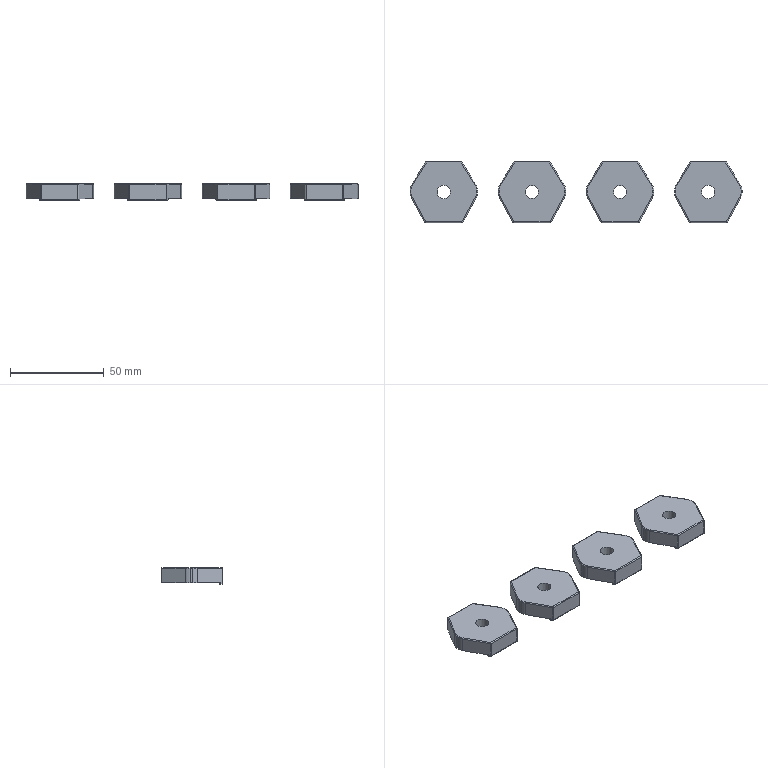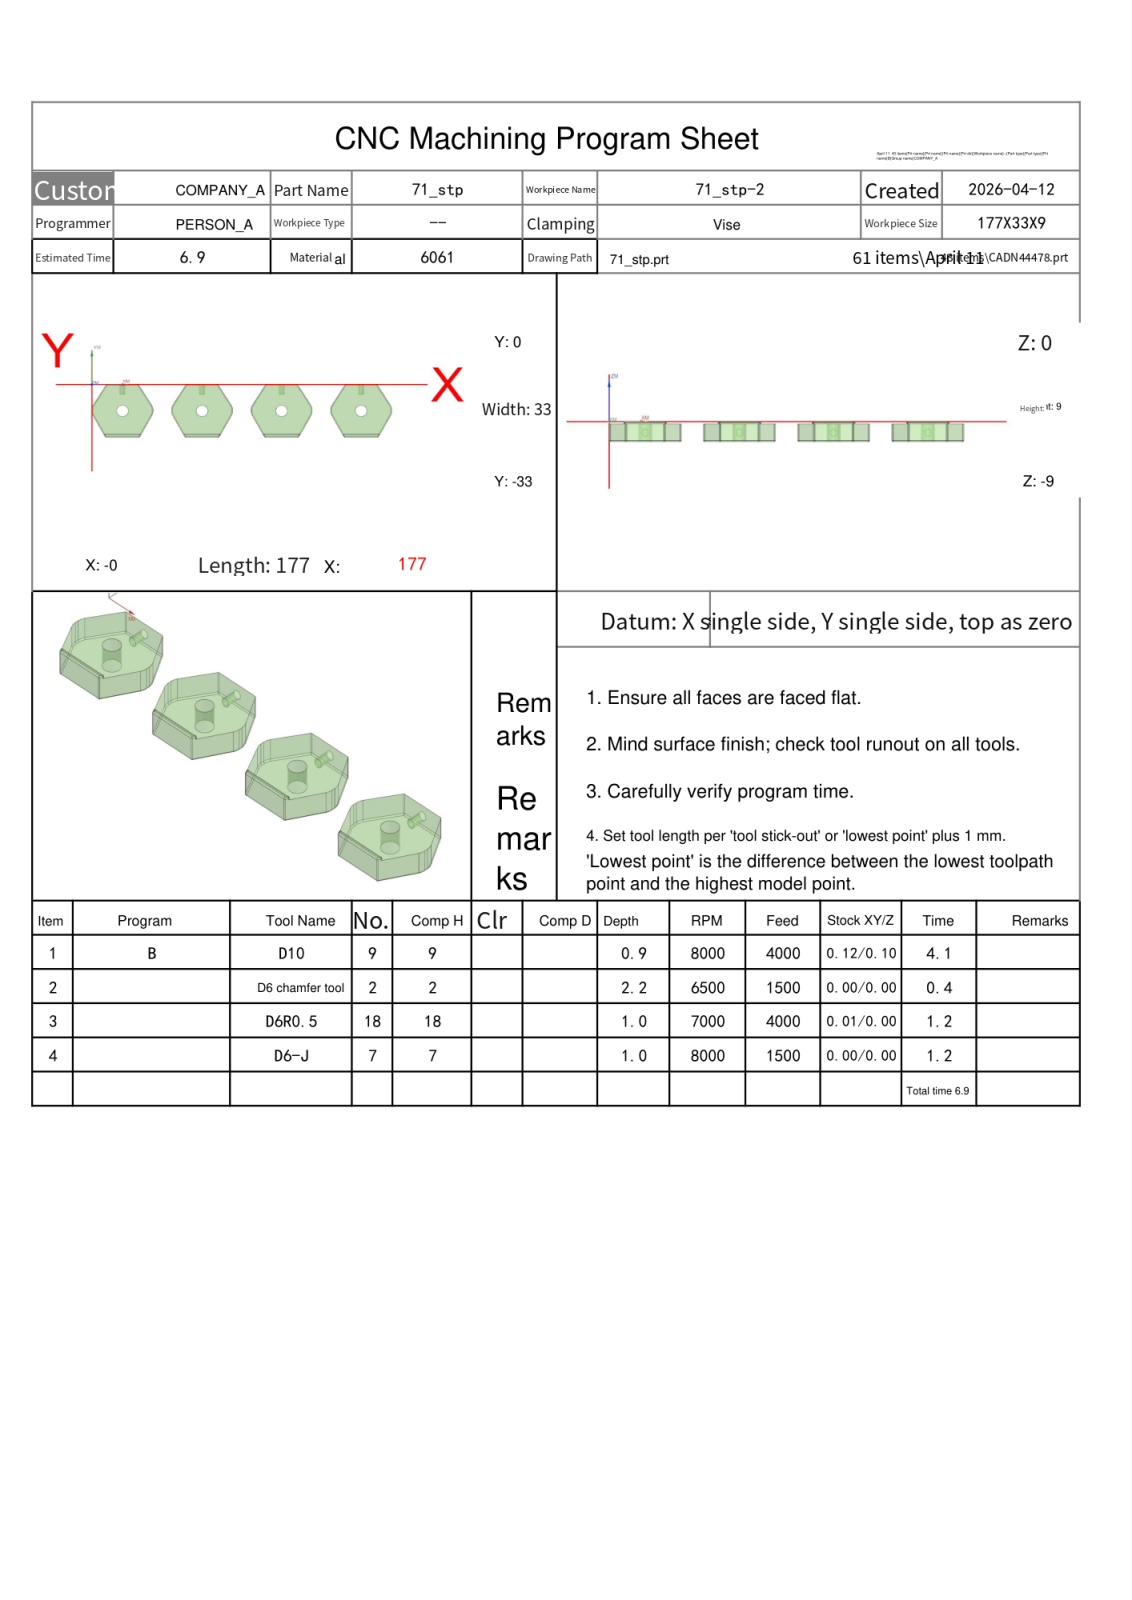NC program | NX | posted by the shop | part box 177 x 33 x 9 mm
Lines 1 to 790 of 12693:
%
O0001
(Machine time: 7.64 MIN)
(===Total Tool:4===)
(T9=D10     D=10.  R=0.   D-  H09 Z=-0.9  )
(T2=D6 chamfer tool   D=6.   R=0.   D-  H02 Z=-2.2  )
(T18=D6R0.5 D=6.   R=0.5  D-  H18 Z=-1.   )
(T7=D6-J    D=6.   R=0.   D7  H07 Z=-1.   )
G80 G90 G17 G49 G40
G91 G28 Z0
M01
N1 T09 M06
(D10  D=10. R=0. H=09 ce=0.12 di=0.10)
G00 G90 G54 X2.999 Y-44.977 M03 S8000
G43 H09 Z50.
M08
Z1.1
G01 X2.983 Y-44.878 Z.476 F4000.
X2.967 Y-44.78 Z.228
X2.951 Y-44.681 Z.046
X2.935 Y-44.582 Z-.1
X2.919 Y-44.484 Z-.223
X2.903 Y-44.385 Z-.328
X2.887 Y-44.286 Z-.42
X2.871 Y-44.187 Z-.5
X2.855 Y-44.089 Z-.57
X2.839 Y-43.99 Z-.632
X2.823 Y-43.891 Z-.686
X2.807 Y-43.793 Z-.733
X2.791 Y-43.694 Z-.774
X2.775 Y-43.595 Z-.808
X2.759 Y-43.496 Z-.836
X2.743 Y-43.398 Z-.86
X2.727 Y-43.299 Z-.877
X2.711 Y-43.2 Z-.89
X2.695 Y-43.102 Z-.897
X2.679 Y-43.003 Z-.9
X2.341 Y-40.918
G03 X2.015 Y-40.524 I-.503 J-.084
X-1.298 Y-40.075 I-3.646 J-14.465
G02 X-7.443 Y-35.315 I.453 J6.931
X-8.402 Y-29.468 I18.063 J5.966
X-8.502 Y-21.143 I348.001 J8.325
X-8.5 Y-19.919 I348.1 J0.0
G01 X-8.479 Y-.331
G02 X-4.048 Y5.824 I6.771 J-.202
X1.676 Y6.882 I5.966 J-16.272
X10.56 Y7.012 I8.884 J-303.294
X13.275 Y7. I0.0 J-303.424
G01 X178.168 Y6.979
G02 X184.324 Y2.548 I-.201 J-6.771
X185.379 Y-3.128 I-16.176 J-5.943
X185.511 Y-11.758 I-283.613 J-8.63
X185.5 Y-14.226 I-283.744 J0.0
G01 X185.479 Y-32.669
G02 X181.002 Y-38.843 I-6.784 J.209
X175.371 Y-39.879 I-5.914 J16.324
X166.48 Y-40.012 I-8.891 J296.264
X163.723 Y-40. I0.0 J296.398
G01 X3.973 Y-39.981
G02 X-1.045 Y-39.489 I1.445 J40.557
X-6.573 Y-34.602 I1.986 J7.816
X-7.843 Y-28.257 I17.624 J6.825
X-8.015 Y-19.083 I243.397 J9.174
X-8. Y-16.31 I243.57 J0.0
X-8.023 Y-10.712 I662.399 J5.597
X-7.96 Y-1.546 I662.422 J0.0
X-3.545 Y4.807 I7.632 J-.592
X2.639 Y6.292 I6.869 J-14.988
X10.363 Y6.506 I7.723 J-139.762
X11.935 Y6.497 I0.0 J-139.976
G01 X176.554 Y6.483
G02 X183.307 Y2.045 I-.199 J-7.661
X184.793 Y-4.139 I-14.987 J-6.87
X185.006 Y-11.881 I-140.304 J-7.742
X184.998 Y-13.435 I-140.517 J0.0
G01 X184.973 Y-31.254
G02 X180.544 Y-37.808 I-7.646 J.394
X174.359 Y-39.292 I-6.869 J14.993
X166.66 Y-39.505 I-7.7 J139.145
X165.114 Y-39.497 I0.0 J139.358
G01 X5.264 Y-39.482
X5.246
G02 X.19 Y-39.041 I0.0 J29.189
X-5.953 Y-33.62 I2.194 J8.678
X-7.301 Y-27.14 I18.598 J7.251
X-7.513 Y-18.286 I185.441 J8.854
X-7.498 Y-15.994 I185.652 J0.0
X-7.515 Y-11.215 I688.153 J4.779
X-7.467 Y-3.095 I688.169 J0.0
X-2.337 Y4.277 I8.552 J-.481
X4.206 Y5.779 I7.342 J-16.98
X13.567 Y6.019 I9.361 J-182.724
X16.301 Y5.998 I0.0 J-182.964
G01 X175.251 Y5.975
G02 X182.777 Y.837 I-.329 J-8.564
X184.279 Y-5.706 I-16.971 J-7.34
X184.507 Y-13.95 I-149.379 J-8.244
X184.497 Y-15.651 I-149.606 J0.0
X184.518 Y-21.237 I-740.341 J-5.586
X184.467 Y-29.9 I-740.362 J0.0
X179.336 Y-37.278 I-8.552 J.476
X172.793 Y-38.779 I-7.342 J16.983
X164.551 Y-39.006 I-8.242 J149.56
X162.848 Y-38.997 I0.0 J149.786
G01 X6.045 Y-38.976
G02 X5.735 Y-38.978 I-.31 J23.836
X1.174 Y-38.538 I0.0 J23.838
X-5.398 Y-32.643 I2.434 J9.325
X-6.795 Y-25.763 I20.244 J7.691
X-7.01 Y-16.708 I190.652 J9.054
X-6.998 Y-14.566 I190.866 J0.0
X-7.023 Y-10.771 I283.282 J3.796
X-6.946 Y-4.168 I283.307 J0.0
X-1.267 Y3.754 I9.248 J-.633
X5.583 Y5.271 I7.719 J-18.63
X15.455 Y5.519 I9.872 J-196.404
X18.328 Y5.498 I0.0 J-196.652
G01 X173.878 Y5.474
G02 X182.254 Y-.234 I-.197 J-9.29
X183.771 Y-7.083 I-18.633 J-7.72
X184.02 Y-16.957 I-196.292 J-9.874
X183.999 Y-19.829 I-196.54 J0.0
X184.018 Y-22.925 I-242.679 J-3.096
X183.947 Y-28.827 I-242.699 J0.0
X178.266 Y-36.755 I-9.248 J.628
X171.416 Y-38.271 I-7.719 J18.634
X162.353 Y-38.511 I-9.063 J171.072
X160.121 Y-38.497 I0.0 J171.311
G01 X6.771 Y-38.473
G02 X6.295 Y-38.479 I-.475 J19.171
X1.668 Y-37.912 I0.0 J19.177
X-4.818 Y-31.828 I3.03 J9.73
X-6.288 Y-24.557 I21.372 J8.103
X-6.51 Y-15.243 I195.457 J9.314
X-6.497 Y-13.06 I195.679 J0.0
X-6.523 Y-10.401 I136.336 J2.659
X-6.421 Y-5.113 I136.362 J0.0
X-.316 Y3.221 I9.807 J-.781
X6.683 Y4.754 I7.994 J-19.754
X16.245 Y5.014 I9.562 J-176.079
X18.678 Y4.997 I0.0 J-176.339
G01 X172.428 Y4.979
X172.54 Y4.98
G02 X181.741 Y-1.229 I0.0 J-9.922
X183.255 Y-8.183 I-19.865 J-7.965
X183.504 Y-16.918 I-152.78 J-8.735
X183.496 Y-18.528 I-153.03 J0.0
X183.517 Y-21.7 I-234.551 J-3.172
X183.442 Y-27.627 I-234.573 J0.0
X177.316 Y-36.221 I-9.835 J.53
X170.665 Y-37.73 I-7.906 J19.433
G01 X170.23 Y-37.908
X168.75 Y-38.12
X148.967 Y-38.102
G03 X141.002 Y-37.999 I-7.965 J-306.286
G01 X140.793
X122.594
X121.75 Y-38.12
X101.967 Y-38.102
G03 X94.002 Y-37.999 I-7.965 J-306.286
G01 X93.793
X75.594
X74.75 Y-38.12
X54.967 Y-38.102
G03 X47.002 Y-37.999 I-7.965 J-306.286
G01 X46.793
X28.827
X27.701 Y-38.12
X7.98 Y-38.097
G02 X3.013 Y-37.547 I.551 J27.664
X-4.209 Y-31.153 I2.65 J10.269
X-5.749 Y-23.89 I21.36 J8.324
X-6.003 Y-14.903 I159.295 J8.987
X-5.995 Y-13.295 I159.548 J0.0
X-6.021 Y-10.976 I103.239 J2.319
X-5.905 Y-6.098 I103.265 J0.0
X.446 Y2.637 I10.264 J-.787
X7.688 Y4.239 I8.311 J-20.407
X17.336 Y4.512 I9.648 J-170.4
X19.633 Y4.496 I0.0 J-170.672
G01 X171.233 Y4.477
X171.375 Y4.478
G02 X177.909 Y2.305 I0.0 J-10.911
X181.905 Y-4.091 I-7.726 J-9.273
X182.894 Y-11.962 I-33.227 J-8.171
X183.008 Y-20.31 I-303.936 J-8.348
X182.948 Y-26.36 I-304.05 J0.0
X176.37 Y-35.718 I-10.37 J.299
X172.083 Y-36.949 I-8.422 J21.239
X170.59 Y-37.753 I-2.913 J3.626
G03 X172.076 Y-36.938 I-1.262 J4.067
G02 X175.512 Y-35.577 I54.848 J-133.461
G03 X181.352 Y-30.069 I-3.976 J10.064
X182.495 Y-24.264 I-15.063 J5.981
X182.606 Y-18.571 I-145.553 J5.693
X182.306 Y-9.222 I-145.665 J0.0
X180.652 Y-2.251 I-20.486 J-1.178
X172.333 Y3.752 I-9.484 J-4.378
X166.206 Y4.1 I-6.127 J-53.718
X165.147 Y4.089 I0.0 J-54.067
G01 X14.497 Y4.071
G03 X13.773 Y4.076 I-.724 J-63.063
X5.323 Y3.507 I0.0 J-63.067
X-1.236 Y.96 I1.922 J-14.668
X-5.252 Y-6.167 I6.416 J-8.31
X-5.599 Y-12.289 I53.869 J-6.122
X-5.585 Y-13.503 I54.216 J0.0
X-5.604 Y-15.59 I112.421 J-2.086
X-5.227 Y-24.792 I112.441 J0.0
X-3.289 Y-31.736 I18.463 J1.411
X4.272 Y-37.136 I9.382 J5.144
G01 X5.596 Y-37.394
G03 X7.1 Y-37.991 I2.82 J4.917
G01 X8.296 Y-38.12
G02 X5.249 Y-37.216 I.134 J6.039
X1.297 Y-35.394 I8.581 J23.816
X-3.815 Y-28.415 I6.703 J10.271
X-4.96 Y-20.468 I30.583 J8.466
X-5.093 Y-14.834 I119.663 J5.634
X-4.913 Y-8.274 I119.796 J0.0
X-2.854 Y-1.984 I12.372 J-.569
X3.688 Y2.404 I9.564 J-7.188
X11.596 Y3.474 I8.331 J-31.79
X21.983 Y3.604 I10.387 J-416.328
X24.345 Y3.597 I0.0 J-416.458
G01 X166.494 Y3.571
G02 X167.073 Y3.577 I.579 J-29.148
X172.855 Y2.998 I0.0 J-29.154
X180.42 Y-3.792 I-2.576 J-10.479
X181.884 Y-11.371 I-23.426 J-8.454
X182.097 Y-18.246 I-110.74 J-6.875
X181.893 Y-24.962 I-110.953 J0.0
X179.522 Y-31.495 I-12.013 J.665
X174.635 Y-35.168 I-10.241 J8.537
G03 X173.061 Y-35.976 I3.524 J-8.798
G02 X172.023 Y-36.977 I-2.965 J2.038
G03 X173.123 Y-35.898 I-2.036 J3.177
G02 X175.777 Y-34.116 I18.901 J-25.281
G03 X181.229 Y-25.549 I-6.539 J10.18
X181.676 Y-18.85 I-49.994 J6.7
X181.654 Y-17.37 I-50.441 J0.0
X181.661 Y-16.477 I-59.649 J.893
X181.062 Y-8.049 I-59.655 J0.0
X178.341 Y-1.333 I-14.574 J-1.997
X171.465 Y2.638 I-8.693 J-7.113
X164.962 Y3.172 I-6.503 J-39.342
X164.494 Y3.169 I0.0 J-39.876
G01 X156.594 Y3.197
X16.595 Y3.175
G03 X15.724 Y3.18 I-.871 J-70.328
X7.017 Y2.639 I0.0 J-70.333
X.346 Y.221 I1.877 J-15.586
X-4.137 Y-7.035 I6.51 J-9.035
X-4.668 Y-13.627 I40.636 J-6.591
X-4.656 Y-14.606 I41.167 J0.0
X-4.672 Y-16.079 I71.417 J-1.472
X-4.151 Y-24.685 I71.432 J0.0
X-1.691 Y-31.597 I16.288 J1.903
X3.606 Y-35.938 I10.684 J7.635
G01 X4.041 Y-36.169
G03 X5.523 Y-37.351 I4.255 J3.816
G02 X3.899 Y-36.024 I3.033 J5.368
X.791 Y-33.441 I37.021 J47.721
X-3.361 Y-25.39 I10.851 J10.691
X-4.126 Y-16.792 I47.911 J8.598
X-4.125 Y-16.435 I48.676 J0.0
X-4.159 Y-14.632 I48.497 J1.803
X-3.738 Y-8.254 I48.53 J0.0
X.296 Y-.907 I11.423 J-1.49
X7.196 Y1.997 I9.133 J-12.052
X15.87 Y2.658 I8.674 J-56.569
X16.312 Y2.656 I0.0 J-57.23
G01 X26.812 Y2.697
X163.262 Y2.677
G02 X163.975 Y2.683 I.713 J-43.732
X170.586 Y2.18 I0.0 J-43.738
X179.634 Y-5.464 I-1.759 J-11.26
X180.998 Y-13.166 I-25.606 J-8.506
X181.153 Y-17.725 I-67.093 J-4.558
X180.859 Y-24.004 I-67.248 J0.0
X177.617 Y-31.512 I-12.997 J1.158
X173.991 Y-34.606 I-20.547 J20.406
X173.085 Y-35.944 I-22.376 J14.182
G03 X174.036 Y-34.512 I-12.25 J9.168
G02 X176.644 Y-31.87 I75.901 J-72.316
G03 X180.376 Y-23.523 I-10.834 J9.853
X180.722 Y-17.37 I-54.613 J6.154
X180.114 Y-9.217 I-54.959 J0.0
X177.33 Y-2.489 I-14.701 J-2.143
X170.339 Y1.614 I-9.142 J-7.571
X163.076 Y2.268 I-7.264 J-39.967
X162.529 Y2.265 I0.0 J-40.622
G01 X154.73 Y2.296
X18.38 Y2.276
G03 X17.47 Y2.281 I-.909 J-75.647
X8.601 Y1.76 I0.0 J-75.652
X1.673 Y-.668 I1.832 J-16.323
X-3.082 Y-8.039 I6.693 J-9.537
X-3.719 Y-14.822 I35.792 J-6.782
X-3.703 Y-15.899 I36.429 J0.0
X-3.709 Y-16.661 I46.333 J-.763
X-2.934 Y-25.101 I46.34 J0.0
X2.353 Y-34.109 I15.234 J2.886
G01 X3.205 Y-34.898
G03 X4.041 Y-36.169 I43.152 J27.457
X2.644 Y-34.08 I-92.584 J-60.397
G02 X-.732 Y-29.325 I19.138 J17.163
X-2.922 Y-21.003 I20.681 J9.89
X-3.183 Y-15.924 I49.234 J5.079
X-2.824 Y-9.976 I49.496 J0.0
X.138 Y-3.142 I12.816 J-1.497
X6.994 Y.753 I9.738 J-9.16
X15.425 Y1.701 I8.651 J-38.953
X26.641 Y1.799 I11.217 J-644.487
X28.474 Y1.796 I0.0 J-644.585
G01 X161.374 Y1.773
G02 X162.031 Y1.778 I.657 J-46.646
X169.146 Y1.232 I0.0 J-46.651
X176.333 Y-2.622 I-1.83 J-12.044
X179.475 Y-9.468 I-11.369 J-9.36
X180.182 Y-17.448 I-44.681 J-7.98
X179.748 Y-23.705 I-45.388 J0.0
X175.437 Y-32.184 I-15.638 J2.616
G03 X174.589 Y-33.235 I2.992 J-3.279
G02 X173.91 Y-34.695 I-11.987 J4.693
G03 X174.773 Y-32.815 I-23.701 J12.019
X177.173 Y-29.217 I-129.625 J89.061
X179.572 Y-20.98 I-16.704 J9.333
X179.736 Y-17.303 I-41. J3.676
X179.005 Y-9.58 I-41.164 J0.0
X175.455 Y-2.637 I-13.442 J-2.494
X168.428 Y.785 I-9.036 J-9.629
X160.713 Y1.378 I-7.715 J-49.884
X159.959 Y1.372 I0.0 J-50.477
G01 X19.459 Y1.371
G03 X18.663 Y1.375 I-.796 J-71.797
X9.683 Y.812 I0.0 J-71.802
X2.778 Y-1.677 I2.002 J-16.377
X-2.056 Y-9.082 I6.995 J-9.848
X-2.741 Y-15.815 I32.781 J-6.733
X-2.696 Y-17.534 I33.465 J0.0
X-1.363 Y-26.453 I31.31 J.124
X2.204 Y-32.814 I20.036 J7.053
G02 X2.814 Y-34.176 I-4.125 J-2.666
G01 X3.147 Y-34.791
G02 X2.134 Y-32.457 I15.644 J8.175
X-.24 Y-27.712 I51.039 J28.512
X-2.114 Y-18.085 I27.203 J10.291
X-2.187 Y-15.964 I30.872 J2.121
X-1.522 Y-9.583 I30.945 J0.0
X6.704 Y-.627 I11.874 J-2.65
X14.717 Y.709 I8.815 J-28.186
X26.129 Y.914 I11.412 J-316.656
X29.564 Y.896 I0.0 J-316.862
G01 X159.364 Y.873
G02 X160.131 Y.879 I.767 J-50.629
X167.784 Y.297 I0.0 J-50.635
X174.891 Y-3.237 I-1.952 J-12.837
X178.46 Y-10.305 I-10.511 J-9.743
X179.173 Y-17.3 I-33.942 J-6.994
X178.573 Y-23.719 I-34.656 J0.0
X175.85 Y-30.133 I-18.897 J4.238
G03 X174.859 Y-31.829 I26.025 J-16.35
G01 X174.594 Y-33.213
G02 X175.054 Y-31.184 I11.414 J-1.522
G03 X177.085 Y-26.841 I-101.382 J50.046
X178.7 Y-17.87 I-24.1 J8.971
X178.692 Y-17.234 I-25.715 J0.0
X178.699 Y-16.643 I-26.433 J.591
X177.404 Y-8.47 I-26.439 J0.0
X168.591 Y-.48 I-11.654 J-3.999
X161.26 Y.408 I-7.592 J-31.958
X151.369 Y.496 I-9.892 J-554.678
G01 X150.361 Y.495
X21.361 Y.474
G03 X20.381 Y.48 I-.98 J-77.222
X11.084 Y-.081 I0.0 J-77.228
X4.016 Y-2.569 I2.013 J-17.004
X-1.089 Y-10.326 I7.087 J-10.222
X-1.718 Y-16.593 I30.919 J-6.267
X-1.502 Y-20.276 I31.548 J0.0
X1.684 Y-30.66 I26.835 J2.554
G01 X2.174 Y-31.724
X2.295 Y-32.826
G03 X1.45 Y-29.34 I-9.727 J-.512
G02 X-1.127 Y-16.735 I29.545 J12.605
X-.703 Y-11.536 I32.121 J0.0
X3.939 Y-3.634 I12.465 J-2.007
X11.113 Y-.728 I9.57 J-13.32
X20.119 Y-.05 I9.006 J-59.481
G01 X20.428 Y-.051
X31.478 Y-.005
X157.578 Y-.027
G02 X158.371 Y-.022 I.793 J-54.817
X166.349 Y-.605 I0.0 J-54.823
X173.478 Y-3.898 I-1.993 J-13.677
X177.425 Y-11.098 I-9.767 J-10.036
X178.13 Y-17.332 I-27.182 J-6.234
X177.001 Y-25.188 I-27.887 J0.0
X175.015 Y-30.091 I-57.448 J20.412
G01 X174.801 Y-30.773
X174.846 Y-31.922
G02 X174.798 Y-31.159 I6.007 J.763
X175.311 Y-28.721 I6.055 J0.0
G03 X177.407 Y-21.017 I-30.9 J12.544
X177.656 Y-17.413 I-25.968 J3.603
X176.622 Y-10.125 I-26.217 J0.0
X167.514 Y-1.452 I-12.114 J-3.604
X159.891 Y-.5 I-7.916 J-32.388
X150.001 Y-.403 I-9.889 J-506.509
X148.591 Y-.405 I0.0 J-506.605
G01 X22.992 Y-.425
G03 X22.049 Y-.42 I-.942 J-84.711
X12.761 Y-.931 I0.0 J-84.716
X5.445 Y-3.321 I1.892 J-18.178
X-.062 Y-11.33 I6.796 J-10.571
X-.651 Y-17.065 I27.608 J-5.735
X-.061 Y-22.801 I28.197 J0.0
X1.937 Y-29.503 I45.841 J10.022
G02 X2.243 Y-30.684 I-13.363 J-4.088
G03 X2.153 Y-31.535 I4.197 J-.872
G02 X2.263 Y-30.434 I8.487 J-.29
G03 X1.588 Y-27.208 I-14.614 J-1.374
G02 X-.035 Y-16.646 I33.55 J10.562
X-.014 Y-15.417 I35.173 J0.0
X2.099 Y-7.837 I16.068 J-.393
X9.464 Y-2.339 I10.962 J-7.004
X17.845 Y-1.072 I9.093 J-31.785
X29.23 Y-.891 I11.386 J-358.936
X32.442 Y-.906 I0.0 J-359.117
G01 X155.842 Y-.927
G02 X156.675 Y-.921 I.832 J-59.306
X164.915 Y-1.497 I0.0 J-59.312
X172.083 Y-4.585 I-2. J-14.504
X176.409 Y-12.045 I-9.139 J-10.284
X177.018 Y-17.672 I-25.701 J-5.627
X175.567 Y-26.291 I-26.31 J0.0
G03 X174.584 Y-29.794 I20.848 J-7.738
G02 X174.8 Y-30.768 I-19.875 J-4.934
G03 X174.57 Y-29.809 I-7.94 J-1.405
G02 X174.999 Y-27.07 I8.982 J-.005
G03 X176.512 Y-18.802 I-35.158 J10.706
X176.56 Y-17.4 I-20.597 J1.403
X175.048 Y-9.646 I-20.645 J0.0
X166.56 Y-2.446 I-11.673 J-5.159
X158.498 Y-1.404 I-8.301 J-32.506
X148.638 Y-1.305 I-9.86 J-489.498
X147.449 Y-1.306 I0.0 J-489.597
G01 X23.699 Y-1.332
G03 X22.855 Y-1.327 I-.844 J-74.942
X13.375 Y-1.929 I0.0 J-74.947
X6.092 Y-4.568 I2.152 J-17.306
X.862 Y-12.86 I7.442 J-10.489
X.455 Y-17.54 I26.663 J-4.68
X1.172 Y-23.731 I27.071 J0.0
G02 X2.391 Y-28.925 I-231.375 J-57.023
X2.466 Y-29.389 I-1.387 J-.464
X2.353 Y-29.954 I-1.463 J0.0
G01 X2.256 Y-30.597
G02 X2.507 Y-29.516 I4.557 J-.489
G03 X2.521 Y-28.956 I-10.904 J.56
X2.193 Y-26.298 I-10.919 J0.0
G02 X1.047 Y-17.952 I44.306 J10.336
X1.027 Y-17.115 I17.692 J.837
X2.556 Y-9.918 I17.712 J0.0
X10.172 Y-3.408 I11.481 J-5.723
X18.078 Y-2.033 I9.028 J-28.498
X28.328 Y-1.799 I10.249 J-224.12
X30.374 Y-1.808 I0.0 J-224.354
G01 X154.674 Y-1.832
G02 X155.343 Y-1.828 I.669 J-59.846
X163.647 Y-2.407 I0.0 J-59.85
X170.944 Y-5.486 I-2.045 J-15.035
X175.446 Y-13.329 I-8.969 J-10.362
X175.897 Y-18.082 I-24.854 J-4.753
X175.136 Y-24.239 I-25.304 J0.0
G03 X174.259 Y-28.664 I31.943 J-8.635
G01 X174.25 Y-28.791
G03 X174.435 Y-29.347 I.928 J0.0
G01 X174.585 Y-29.877
G03 X174.257 Y-29.019 I-2.714 J-.547
G02 X174.182 Y-27.955 I7.543 J1.064
X174.393 Y-26.174 I7.618 J0.0
G03 X175.4 Y-19.095 I-49.35 J10.63
X175.443 Y-17.826 I-18.652 J1.269
X173.807 Y-10.178 I-18.695 J0.0
X165.7 Y-3.46 I-11.538 J-5.674
X157.551 Y-2.323 I-8.52 J-31.284
X147.402 Y-2.2 I-10.149 J-419.778
X145.052 Y-2.207 I0.0 J-419.901
G01 X25.852 Y-2.226
G03 X24.852 Y-2.22 I-1. J-89.082
X15.271 Y-2.737 I0.0 J-89.088
X7.88 Y-5.066 I1.981 J-19.182
X1.91 Y-13.921 I6.654 J-10.925
X1.564 Y-18.153 I25.706 J-4.232
X2.024 Y-23.023 I26.052 J0.0
G02 X2.803 Y-28.055 I-57.925 J-11.551
X2.824 Y-28.381 I-2.591 J-.326
X2.454 Y-29.721 I-2.612 J0.0
G03 X3.011 Y-27.432 I-4.417 J2.289
X2.96 Y-26.717 I-4.975 J0.0
G01 X2.249 Y-20.6
G02 X2.124 Y-18.339 I20.347 J2.26
X2.992 Y-12.44 I20.472 J0.0
X10.9 Y-4.475 I12.04 J-4.046
X18.831 Y-2.969 I9.196 J-26.797
X29.258 Y-2.698 I10.427 J-200.451
X31.375 Y-2.709 I0.0 J-200.722
G01 X152.925 Y-2.73
G02 X153.758 Y-2.724 I.832 J-63.518
X162.448 Y-3.322 I0.0 J-63.524
X169.731 Y-6.319 I-2.11 J-15.472
X174.45 Y-14.641 I-8.666 J-10.414
X174.767 Y-18.654 I-25.202 J-4.012
X174.35 Y-23.249 I-25.519 J0.0
G03 X173.814 Y-27.683 I29.929 J-5.868
X173.894 Y-28.382 I9.957 J.787
G01 X174.31 Y-29.123
G02 X173.632 Y-26.973 I3.07 J2.15
X173.655 Y-26.554 I3.747 J0.0
X174.188 Y-21.222 I123.352 J-9.623
G03 X174.324 Y-18.852 I-20.612 J2.37
X173.382 Y-12.673 I-20.748 J0.0
X164.803 Y-4.458 I-12.175 J-4.128
X156.866 Y-3.253 I-8.567 J-29.684
X146.466 Y-3.095 I-10.4 J-342.826
X143.618 Y-3.107 I0.0 J-342.983
G01 X27.318 Y-3.126
G03 X26.251 Y-3.119 I-1.068 J-91.707
X16.487 Y-3.64 I0.0 J-91.714
X8.995 Y-5.988 I1.993 J-19.493
X2.962 Y-15.051 I6.616 J-10.943
X2.667 Y-19. I26.355 J-3.949
X2.922 Y-22.674 I26.649 J0.0
G02 X3.287 Y-27.427 I-32.198 J-4.862
X3.115 Y-28.386 I-2.769 J.001
G03 X2.808 Y-28.9 I1.516 J-1.253
G02 X3.242 Y-28.169 I4.668 J-2.278
G03 X3.587 Y-25.839 I-7.701 J2.331
X3.541 Y-24.978 I-8.046 J0.0
G02 X3.244 Y-18.424 I79.002 J6.865
G01 Y-18.408
G02 X5.376 Y-10.607 I15.338 J0.0
X12.668 Y-5.165 I11.133 J-7.309
X21.085 Y-3.807 I9.349 J-31.187
X33.085 Y-3.588 I12. J-329.031
X36.682 Y-3.608 I0.0 J-329.25
G01 X151.432 Y-3.63
G02 X152.249 Y-3.625 I.817 J-68.013
X161.007 Y-4.191 I0.0 J-68.018
X168.294 Y-6.983 I-2.059 J-16.28
X173.358 Y-15.579 I-8.051 J-10.531
X173.654 Y-19.602 I-27.205 J-4.024
X173.448 Y-22.955 I-27.501 J0.0
G03 X173.259 Y-25.678 I19.442 J-2.723
X173.323 Y-27.269 I19.632 J0.0
X173.79 Y-28.195 I1.24 J.044
G01 X173.888 Y-28.37
G03 X173.447 Y-27.819 I-3.185 J-2.096
G02 X172.998 Y-25.564 I5.445 J2.255
X173.012 Y-25.157 I5.894 J0.0
G03 X173.199 Y-19.122 I-171.194 J8.326
G01 X173.2 Y-18.992
G03 X171.115 Y-11.031 I-16.242 J0.0
X163.434 Y-5.301 I-11.162 J-6.951
X155.387 Y-4.146 I-8.65 J-31.643
X144.901 Y-3.998 I-10.487 J-371.111
X142.189 Y-4.008 I0.0 J-371.259
G01 X28.539 Y-4.027
G03 X27.531 Y-4.022 I-1.008 J-93.419
X17.758 Y-4.534 I0.0 J-93.424
X10.245 Y-6.827 I2. J-20.009
X4.025 Y-16.122 I6.471 J-11.06
X3.732 Y-20.195 I28.172 J-4.072
X3.806 Y-22.256 I28.465 J0.0
G02 X3.913 Y-24.547 I-24.67 J-2.291
X3.795 Y-26.962 I-24.776 J0.0
X3.128 Y-28.369 I-2.117 J.142
G03 X4.17 Y-25.794 I-2.949 J2.691
X4.281 Y-21.921 I-67.233 J3.873
X4.261 Y-20.286 I-67.345 J0.0
G02 X4.259 Y-19.979 I17.921 J.308
X5.702 Y-12.932 I17.923 J0.0
X13.198 Y-6.288 I11.654 J-5.598
X21.43 Y-4.762 I9.433 J-27.932
X32.337 Y-4.497 I10.906 J-223.678
X34.776 Y-4.51 I0.0 J-223.944
G01 X149.476 Y-4.526
G02 X150.514 Y-4.519 I1.038 J-76.068
X159.554 Y-5.058 I0.0 J-76.075
X166.886 Y-7.684 I-1.982 J-17.083
X172.203 Y-16.174 I-7.529 J-10.625
X172.599 Y-20.833 I-27.241 J-4.659
X172.574 Y-22. I-27.637 J0.0
G03 X172.527 Y-23.486 I23.526 J-1.486
X172.714 Y-26.451 I23.573 J0.0
X173.502 Y-27.884 I2.112 J.228
G02 X172.423 Y-25.734 I2.107 J2.404
X172.182 Y-21.458 I37.852 J4.276
X172.187 Y-20.858 I38.093 J0.0
G01 Y-20.671
G03 X170.814 Y-13.482 I-19.506 J0.0
X162.783 Y-6.369 I-11.778 J-5.208
X154.61 Y-5.071 I-8.871 J-29.486
X143.99 Y-4.896 I-10.62 J-321.327
X141.112 Y-4.909 I0.0 J-321.503
G01 X29.262 Y-4.932
G03 X28.323 Y-4.927 I-.94 J-84.414
X18.386 Y-5.514 I0.0 J-84.419
X10.943 Y-7.99 I2.199 J-19.035
X5.132 Y-16.818 I6.896 J-10.866
X4.674 Y-22.732 I37.951 J-5.914
X4.677 Y-23.255 I38.409 J0.0
G02 X4.68 Y-23.511 I-12.488 J-.256
X4.179 Y-27.013 I-12.491 J0.0
X3.822 Y-27.486 I-.839 J.262
G01 X3.606 Y-27.761
G02 X4.148 Y-27.189 I5.614 J-4.776
G03 X4.967 Y-24.305 I-5.836 J3.217
G02 X5.45 Y-18.534 I176.788 J-11.881
X8.736 Y-10.881 I13.992 J-1.475
X16.041 Y-6.651 I10.703 J-10.064
X25.004 Y-5.541 I9.501 J-39.955
X36.419 Y-5.402 I11.415 J-470.329
X38.952 Y-5.409 I0.0 J-470.467
G01 X148.252 Y-5.427
G02 X149.229 Y-5.421 I.977 J-77.597
X158.331 Y-5.957 I0.0 J-77.604
X165.603 Y-8.479 I-2.01 J-17.539
X171.075 Y-16.817 I-7.303 J-10.758
X171.718 Y-23.18 I-39.26 J-7.184
G03 X172.365 Y-26.705 I10.585 J.12
X172.893 Y-27.226 I.969 J.454
G01 X172.961 Y-27.299
G02 X171.906 Y-25.824 I1.245 J2.004
X171.295 Y-21.918 I17.934 J4.809
G03 X170.099 Y-15.296 I-25.367 J-1.162
X161.728 Y-7.304 I-12.173 J-4.369
X153.909 Y-6.002 I-8.777 J-28.579
X143.647 Y-5.797 I-10.262 J-257.332
X141.112 Y-5.81 I0.0 J-257.537
G01 X30.962 Y-5.829
G03 X29.892 Y-5.823 I-1.069 J-91.342
X19.783 Y-6.384 I0.0 J-91.348
X12.292 Y-8.756 I2.149 J-19.805
X6.236 Y-17.357 I6.696 J-11.147
X5.459 Y-23.293 I47.03 J-9.18
G02 X4.581 Y-26.828 I-9.609 J.509
X3.992 Y-27.358 I-1.497 J1.072
G03 X5.352 Y-25.41 I-1.726 J2.653
X6.221 Y-20.534 I-30.964 J8.034
G02 X8.339 Y-13.8 I17.855 J-1.915
X15.967 Y-7.919 I11.564 J-7.113
X24.38 Y-6.53 I9.503 J-31.377
X36.959 Y-6.287 I12.579 J-325.834
X40.776 Y-6.31 I0.0 J-326.076
G01 X147.326 Y-6.331
G02 X148.176 Y-6.327 I.85 J-75.296
X157.303 Y-6.882 I0.0 J-75.301
X164.727 Y-9.545 I-2.035 J-17.35
X170.01 Y-17.569 I-7.702 J-10.822
X170.948 Y-23.392 I-60.87 J-12.802
G03 X171.943 Y-26.57 I8.051 J.776
G01 X172.556 Y-27.
G02 X171.199 Y-25.331 I1.27 J2.419
X170.223 Y-20.864 I23.366 J7.444
G03 X168.166 Y-14.264 I-19.686 J-2.513
X160.312 Y-8.114 I-11.528 J-6.633
X152.378 Y-6.885 I-8.817 J-30.7
X141.403 Y-6.694 I-10.975 J-315.211
X138.281 Y-6.71 I0.0 J-315.402
G01 X31.931 Y-6.733
G03 X30.986 Y-6.728 I-.945 J-90.718
X21.001 Y-7.279 I0.0 J-90.723
X13.414 Y-9.652 I2.134 J-20.141
X7.273 Y-18.003 I6.869 J-11.485
X6.13 Y-23.724 I90.512 J-21.059
G02 X5.048 Y-26.562 I-7.23 J1.132
G01 X4.5 Y-26.975
G03 X6.109 Y-24.845 I-1.945 J3.142
X7.318 Y-20.033 I-39.622 J12.512
G02 X10.292 Y-13.374 I16.077 J-3.186
X17.814 Y-8.594 I11.189 J-9.301
X26.76 Y-7.369 I9.657 J-37.238
X38.858 Y-7.197 I12.099 J-424.503
X42.208 Y-7.21 I0.0 J-424.675
G01 X146.008 Y-7.232
G02 X146.88 Y-7.227 I.873 J-77.364
X156.085 Y-7.776 I0.0 J-77.369
X163.445 Y-10.328 I-2.057 J-17.824
X168.853 Y-17.827 I-7.59 J-11.173
X170.148 Y-23.265 I-74.079 J-20.513
G03 X171.389 Y-26.283 I7.748 J1.422
G01 X172.003 Y-26.631
X171.34 Y-26.267
G02 X170.01 Y-23.751 I4.425 J3.947
G03 X168.562 Y-18.428 I-406.047 J-107.636
X162.911 Y-10.731 I-13.259 J-3.81
X155.437 Y-8.183 I-9.629 J-16.011
X146.22 Y-7.632 I-9.217 J-76.748
X145.509 Y-7.635 I0.0 J-77.299
G01 X33.259 Y-7.632
G03 X32.246 Y-7.627 I-1.013 J-92.039
X22.08 Y-8.19 I0.0 J-92.045
X14.317 Y-10.665 I2.149 J-20.157
X8.366 Y-18.311 I7.236 J-11.771
X6.85 Y-23.692 I139.391 J-42.171
G02 X5.484 Y-26.379 I-6.519 J1.623
G01 X4.979 Y-26.614
G03 X6.508 Y-25.196 I-.865 J2.465
X7.751 Y-21.989 I-15.243 J7.754
G02 X10.009 Y-16.157 I26.407 J-6.872
X18.302 Y-9.686 I12.29 J-7.201
X26.872 Y-8.323 I9.65 J-33.074
X39.467 Y-8.09 I12.595 J-339.777
X43.218 Y-8.111 I0.0 J-340.011
G01 X145.118 Y-8.136
G02 X145.942 Y-8.131 I.824 J-72.921
X155.292 Y-8.733 I0.0 J-72.926
X162.816 Y-11.542 I-2.173 J-17.299
X167.909 Y-18.626 I-8.566 J-11.532
G01 X169.543 Y-23.754
G03 X170.93 Y-26.157 I5.877 J1.79
G01 X171.577 Y-26.412
G02 X169.94 Y-25.074 I.624 J2.434
X168.565 Y-21.812 I14.712 J8.121
G03 X166.2 Y-16.126 I-26.787 J-7.808
X157.585 Y-9.772 I-12.091 J-7.374
X149.179 Y-8.649 I-9.04 J-35.65
X138.233 Y-8.502 I-10.946 J-407.839
X135.481 Y-8.511 I0.0 J-407.986
G01 X34.431 Y-8.533
G03 X33.504 Y-8.529 I-.927 J-95.21
X23.4 Y-9.066 I0.0 J-95.215
X15.514 Y-11.487 I2.11 J-20.934
X9.359 Y-18.82 I7.409 J-12.469
G01 X7.457 Y-23.951
G02 X5.957 Y-26.215 I-5.311 J1.891
G01 X5.402 Y-26.441
G03 X7.327 Y-24.784 I-1.014 J3.124
X9.279 Y-20.381 I-28.077 J15.083
G02 X13.376 Y-14. I16.211 J-5.903
X21.232 Y-10.082 I11.105 J-12.434
X30.417 Y-9.121 I9.66 J-47.944
X42.381 Y-9.007 I11.964 J-629.325
X44.616 Y-9.011 I0.0 J-629.439
G01 X143.316 Y-9.031
G02 X144.304 Y-9.025 I.987 J-81.488
X153.794 Y-9.58 I0.0 J-81.494
X161.355 Y-12.17 I-2.098 J-18.456
X166.776 Y-18.807 I-8.284 J-12.299
G01 X168.797 Y-23.749
G03 X170.335 Y-25.971 I5.641 J2.264
G01 X170.978 Y-26.191
G02 X169.219 Y-24.904 I.593 J2.655
X167.613 Y-21.772 I14.94 J9.642
G03 X164.727 Y-16.203 I-25.409 J-9.632
X156.087 Y-10.563 I-11.987 J-8.926
X147.216 Y-9.519 I-9.231 J-40.239
X136.296 Y-9.409 I-10.92 J-537.636
X134.467 Y-9.412 I0.0 J-537.747
G01 X35.717 Y-9.433
G03 X34.765 Y-9.429 I-.952 J-98.024
X24.586 Y-9.959 I0.0 J-98.029
X16.631 Y-12.339 I2.145 J-21.656
X10.251 Y-19.444 I7.779 J-13.402
G02 X8.014 Y-24.223 I-88.494 J38.499
X6.553 Y-26.014 I-4.83 J2.449
G01 X6.042 Y-26.18
G03 X6.813 Y-25.902 I-2.26 J7.481
X8.76 Y-23.515 I-4.024 J5.269
G02 X11.399 Y-18.489 I110.78 J-54.971
X21.275 Y-11.239 I13.616 J-8.195
X30.132 Y-10.076 I9.745 J-39.913
X41.965 Y-9.901 I11.834 J-400.105
X44.93 Y-9.912 I0.0 J-400.28
G01 X142.08 Y-9.932
G02 X143.02 Y-9.927 I.94 J-85.024
X152.509 Y-10.458 I0.0 J-85.029
X160.24 Y-13.015 I-2.071 J-19.228
X165.827 Y-19.355 I-8.676 J-13.276
G03 X168.242 Y-24.109 I88.18 J41.8
X169.902 Y-25.944 I4.475 J2.382
G01 X170.536 Y-26.033
G02 X168.826 Y-25.191 I.01 J2.177
X166.671 Y-21.836 I11.393 J9.687